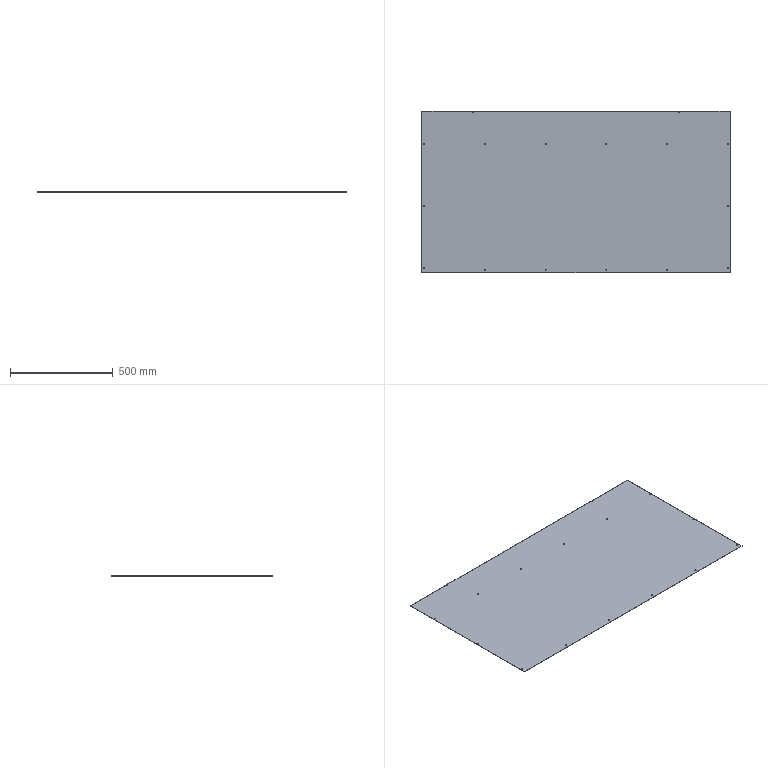Part | STEP file | SX-S22 | 1 solid | 38 faces | box 1498 x 785 x 1.2 mm | volume 1410637 mm3 | cylinder 30 | plane 8 | commonest cylinder face diameters 5.4 x28 10 x2